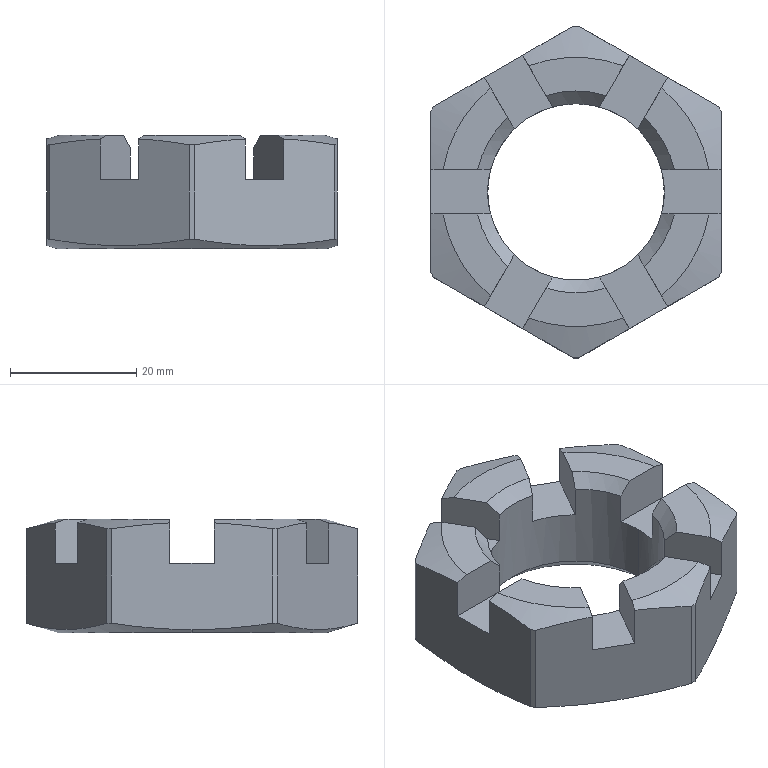Part | STEP file | SHAFT_CAP1V11 | 1 solid | 55 faces | box 46 x 52.616 x 18 mm | volume 18537 mm3 | plane 37 | cone 16 | cylinder 2 | commonest cylinder face diameters 28 x2